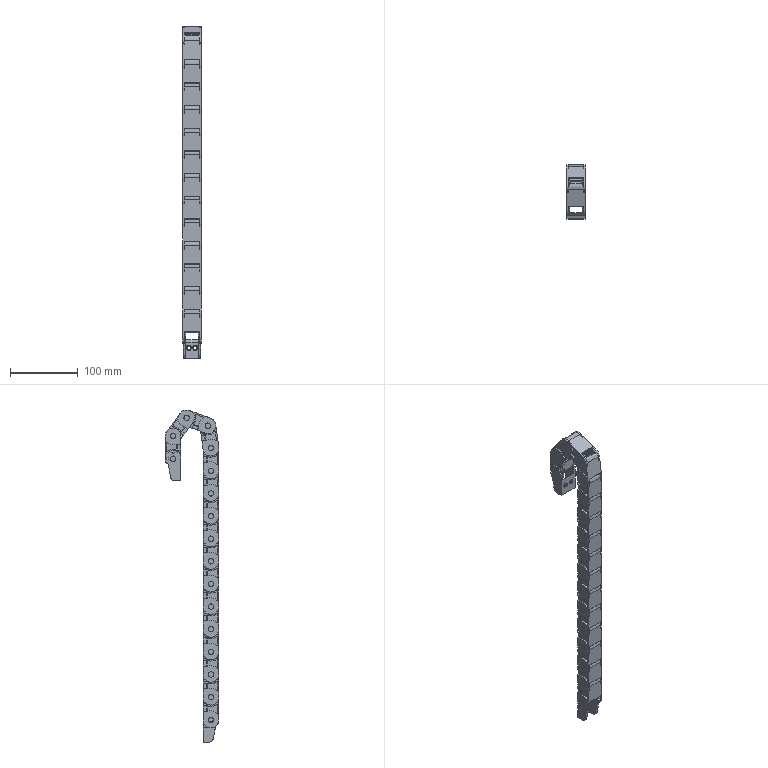Part | SolidWorks | features BaseBody 18 | 18 solids | 2350 faces | box 29.1 x 79.262 x 491.255 mm | volume 146687 mm3 | plane 1340 | cylinder 996 | cone 10 | spline 4 | commonest cylinder face diameters 2 x192 1 x176 0.6 x112 11.94 x96 23.26 x80 24.06 x80